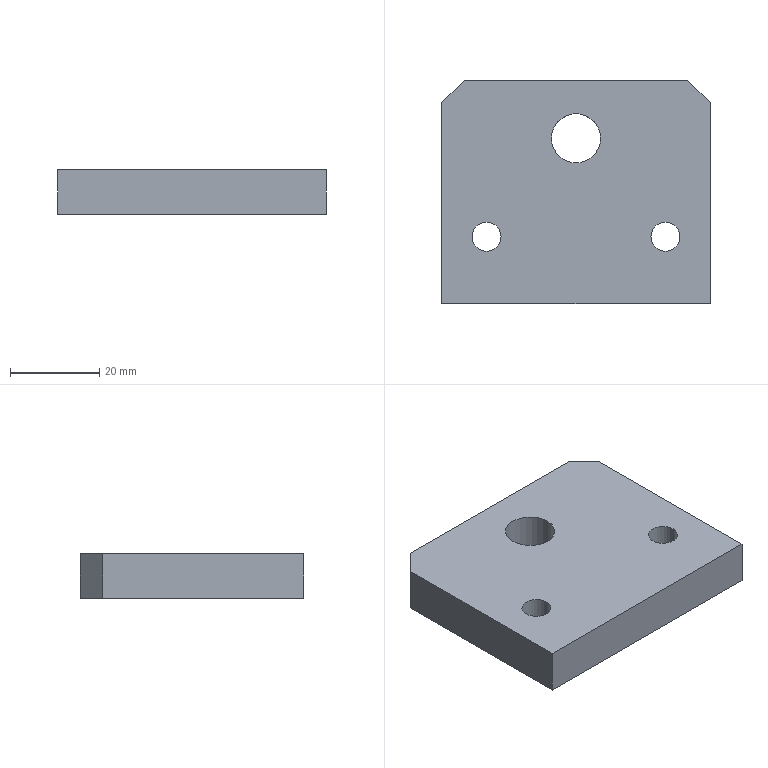Part | SolidWorks | features Cut 2, Chamfer 1, Extrusion 1 | 1 solid | 14 faces | box 60 x 50 x 10 mm | volume 28136 mm3 | plane 8 | cylinder 6 | commonest cylinder face diameters 6.5 x4 11 x2
STEP:
#1=CARTESIAN_POINT('',(-21.994,-12.765,10.));
#2=VERTEX_POINT('',#1);
#3=CARTESIAN_POINT('',(-28.494,-12.765,10.));
#4=VERTEX_POINT('',#3);
#5=CARTESIAN_POINT('',(-25.244,-12.765,10.));
#6=DIRECTION('',(0.,0.,-1.));
#7=DIRECTION('',(-1.,0.,0.));
#8=AXIS2_PLACEMENT_3D('',#5,#6,#7);
#9=CIRCLE('',#8,3.25);
#10=EDGE_CURVE('',#2,#4,#9,.T.);
#11=ORIENTED_EDGE('',*,*,#10,.F.);
#12=CARTESIAN_POINT('',(-21.994,-12.765,0.));
#13=VERTEX_POINT('',#12);
#14=CARTESIAN_POINT('',(-21.994,-12.765,10.));
#15=DIRECTION('',(0.,0.,-1.));
#16=VECTOR('',#15,1000.);
#17=LINE('',#14,#16);
#18=EDGE_CURVE('',#2,#13,#17,.T.);
#19=ORIENTED_EDGE('',*,*,#18,.T.);
#20=CARTESIAN_POINT('',(-28.494,-12.765,0.));
#21=VERTEX_POINT('',#20);
#22=CARTESIAN_POINT('',(-25.244,-12.765,0.));
#23=DIRECTION('',(0.,0.,-1.));
#24=DIRECTION('',(-1.,0.,0.));
#25=AXIS2_PLACEMENT_3D('',#22,#23,#24);
#26=CIRCLE('',#25,3.25);
#27=EDGE_CURVE('',#13,#21,#26,.T.);
#28=ORIENTED_EDGE('',*,*,#27,.T.);
#29=CARTESIAN_POINT('',(-28.494,-12.765,10.));
#30=DIRECTION('',(0.,0.,-1.));
#31=VECTOR('',#30,1000.);
#32=LINE('',#29,#31);
#33=EDGE_CURVE('',#4,#21,#32,.T.);
#34=ORIENTED_EDGE('',*,*,#33,.F.);
#35=EDGE_LOOP('',(#11,#19,#28,#34));
#36=FACE_OUTER_BOUND('',#35,.T.);
#37=CARTESIAN_POINT('',(-25.244,-12.765,10.));
#38=DIRECTION('',(0.,0.,-1.));
#39=DIRECTION('',(-1.,0.,0.));
#40=AXIS2_PLACEMENT_3D('',#37,#38,#39);
#41=CYLINDRICAL_SURFACE('',#40,3.25);
#42=ADVANCED_FACE('',(#36),#41,.F.);
#43=CARTESIAN_POINT('',(18.006,-12.765,10.));
#44=VERTEX_POINT('',#43);
#45=CARTESIAN_POINT('',(11.506,-12.765,10.));
#46=VERTEX_POINT('',#45);
#47=CARTESIAN_POINT('',(14.756,-12.765,10.));
#48=DIRECTION('',(0.,0.,-1.));
#49=DIRECTION('',(-1.,0.,0.));
#50=AXIS2_PLACEMENT_3D('',#47,#48,#49);
#51=CIRCLE('',#50,3.25);
#52=EDGE_CURVE('',#44,#46,#51,.T.);
#53=ORIENTED_EDGE('',*,*,#52,.F.);
#54=CARTESIAN_POINT('',(18.006,-12.765,0.));
#55=VERTEX_POINT('',#54);
#56=CARTESIAN_POINT('',(18.006,-12.765,10.));
#57=DIRECTION('',(0.,0.,-1.));
#58=VECTOR('',#57,1000.);
#59=LINE('',#56,#58);
#60=EDGE_CURVE('',#44,#55,#59,.T.);
#61=ORIENTED_EDGE('',*,*,#60,.T.);
#62=CARTESIAN_POINT('',(11.506,-12.765,0.));
#63=VERTEX_POINT('',#62);
#64=CARTESIAN_POINT('',(14.756,-12.765,0.));
#65=DIRECTION('',(0.,0.,-1.));
#66=DIRECTION('',(-1.,0.,0.));
#67=AXIS2_PLACEMENT_3D('',#64,#65,#66);
#68=CIRCLE('',#67,3.25);
#69=EDGE_CURVE('',#55,#63,#68,.T.);
#70=ORIENTED_EDGE('',*,*,#69,.T.);
#71=CARTESIAN_POINT('',(11.506,-12.765,10.));
#72=DIRECTION('',(0.,0.,-1.));
#73=VECTOR('',#72,1000.);
#74=LINE('',#71,#73);
#75=EDGE_CURVE('',#46,#63,#74,.T.);
#76=ORIENTED_EDGE('',*,*,#75,.F.);
#77=EDGE_LOOP('',(#53,#61,#70,#76));
#78=FACE_OUTER_BOUND('',#77,.T.);
#79=CARTESIAN_POINT('',(14.756,-12.765,10.));
#80=DIRECTION('',(0.,0.,-1.));
#81=DIRECTION('',(-1.,0.,0.));
#82=AXIS2_PLACEMENT_3D('',#79,#80,#81);
#83=CYLINDRICAL_SURFACE('',#82,3.25);
#84=ADVANCED_FACE('',(#78),#83,.F.);
#85=CARTESIAN_POINT('',(-10.744,9.235,10.));
#86=VERTEX_POINT('',#85);
#87=CARTESIAN_POINT('',(0.2561,9.235,10.));
#88=VERTEX_POINT('',#87);
#89=CARTESIAN_POINT('',(-5.244,9.235,10.));
#90=DIRECTION('',(0.,0.,1.));
#91=DIRECTION('',(1.,0.,0.));
#92=AXIS2_PLACEMENT_3D('',#89,#90,#91);
#93=CIRCLE('',#92,5.5);
#94=EDGE_CURVE('',#86,#88,#93,.T.);
#95=ORIENTED_EDGE('',*,*,#94,.T.);
#96=CARTESIAN_POINT('',(0.2561,9.235,0.));
#97=VERTEX_POINT('',#96);
#98=CARTESIAN_POINT('',(0.2561,9.235,18.));
#99=DIRECTION('',(0.,0.,-1.));
#100=VECTOR('',#99,1000.);
#101=LINE('',#98,#100);
#102=EDGE_CURVE('',#88,#97,#101,.T.);
#103=ORIENTED_EDGE('',*,*,#102,.T.);
#104=CARTESIAN_POINT('',(-10.744,9.235,0.));
#105=VERTEX_POINT('',#104);
#106=CARTESIAN_POINT('',(-5.244,9.235,0.));
#107=DIRECTION('',(0.,0.,-1.));
#108=DIRECTION('',(-1.,0.,0.));
#109=AXIS2_PLACEMENT_3D('',#106,#107,#108);
#110=CIRCLE('',#109,5.5);
#111=EDGE_CURVE('',#97,#105,#110,.T.);
#112=ORIENTED_EDGE('',*,*,#111,.T.);
#113=CARTESIAN_POINT('',(-10.744,9.235,18.));
#114=DIRECTION('',(0.,0.,-1.));
#115=VECTOR('',#114,1000.);
#116=LINE('',#113,#115);
#117=EDGE_CURVE('',#86,#105,#116,.T.);
#118=ORIENTED_EDGE('',*,*,#117,.F.);
#119=EDGE_LOOP('',(#95,#103,#112,#118));
#120=FACE_OUTER_BOUND('',#119,.T.);
#121=CARTESIAN_POINT('',(-5.244,9.235,18.));
#122=DIRECTION('',(0.,0.,-1.));
#123=DIRECTION('',(-1.,0.,0.));
#124=AXIS2_PLACEMENT_3D('',#121,#122,#123);
#125=CYLINDRICAL_SURFACE('',#124,5.5);
#126=ADVANCED_FACE('',(#120),#125,.F.);
#127=CARTESIAN_POINT('',(-35.244,17.235,10.));
#128=VERTEX_POINT('',#127);
#129=CARTESIAN_POINT('',(-35.244,-27.765,10.));
#130=VERTEX_POINT('',#129);
#131=CARTESIAN_POINT('',(-35.244,22.235,10.));
#132=DIRECTION('',(0.,-1.,0.));
#133=VECTOR('',#132,1000.);
#134=LINE('',#131,#133);
#135=EDGE_CURVE('',#128,#130,#134,.T.);
#136=ORIENTED_EDGE('',*,*,#135,.F.);
#137=CARTESIAN_POINT('',(-35.244,17.235,0.));
#138=VERTEX_POINT('',#137);
#139=CARTESIAN_POINT('',(-35.244,17.235,10.));
#140=DIRECTION('',(0.,0.,-1.));
#141=VECTOR('',#140,1000.);
#142=LINE('',#139,#141);
#143=EDGE_CURVE('',#128,#138,#142,.T.);
#144=ORIENTED_EDGE('',*,*,#143,.T.);
#145=CARTESIAN_POINT('',(-35.244,-27.765,0.));
#146=VERTEX_POINT('',#145);
#147=CARTESIAN_POINT('',(-35.244,22.235,0.));
#148=DIRECTION('',(0.,-1.,0.));
#149=VECTOR('',#148,1000.);
#150=LINE('',#147,#149);
#151=EDGE_CURVE('',#138,#146,#150,.T.);
#152=ORIENTED_EDGE('',*,*,#151,.T.);
#153=CARTESIAN_POINT('',(-35.244,-27.765,10.));
#154=DIRECTION('',(0.,0.,-1.));
#155=VECTOR('',#154,1000.);
#156=LINE('',#153,#155);
#157=EDGE_CURVE('',#130,#146,#156,.T.);
#158=ORIENTED_EDGE('',*,*,#157,.F.);
#159=EDGE_LOOP('',(#136,#144,#152,#158));
#160=FACE_OUTER_BOUND('',#159,.T.);
#161=CARTESIAN_POINT('',(-35.244,22.235,10.));
#162=DIRECTION('',(1.,0.,0.));
#163=DIRECTION('',(0.,0.,-1.));
#164=AXIS2_PLACEMENT_3D('',#161,#162,#163);
#165=PLANE('',#164);
#166=ADVANCED_FACE('',(#160),#165,.F.);
#167=CARTESIAN_POINT('',(24.756,-27.765,0.));
#168=VERTEX_POINT('',#167);
#169=CARTESIAN_POINT('',(-35.244,-27.765,0.));
#170=DIRECTION('',(1.,0.,0.));
#171=VECTOR('',#170,1000.);
#172=LINE('',#169,#171);
#173=EDGE_CURVE('',#146,#168,#172,.T.);
#174=ORIENTED_EDGE('',*,*,#173,.T.);
#175=CARTESIAN_POINT('',(24.756,-27.765,10.));
#176=VERTEX_POINT('',#175);
#177=CARTESIAN_POINT('',(24.756,-27.765,10.));
#178=DIRECTION('',(0.,0.,-1.));
#179=VECTOR('',#178,1000.);
#180=LINE('',#177,#179);
#181=EDGE_CURVE('',#176,#168,#180,.T.);
#182=ORIENTED_EDGE('',*,*,#181,.F.);
#183=CARTESIAN_POINT('',(-35.244,-27.765,10.));
#184=DIRECTION('',(1.,0.,0.));
#185=VECTOR('',#184,1000.);
#186=LINE('',#183,#185);
#187=EDGE_CURVE('',#130,#176,#186,.T.);
#188=ORIENTED_EDGE('',*,*,#187,.F.);
#189=ORIENTED_EDGE('',*,*,#157,.T.);
#190=EDGE_LOOP('',(#174,#182,#188,#189));
#191=FACE_OUTER_BOUND('',#190,.T.);
#192=CARTESIAN_POINT('',(-35.244,-27.765,10.));
#193=DIRECTION('',(0.,1.,0.));
#194=DIRECTION('',(0.,0.,1.));
#195=AXIS2_PLACEMENT_3D('',#192,#193,#194);
#196=PLANE('',#195);
#197=ADVANCED_FACE('',(#191),#196,.F.);
#198=CARTESIAN_POINT('',(24.756,17.235,0.));
#199=VERTEX_POINT('',#198);
#200=CARTESIAN_POINT('',(24.756,22.235,0.));
#201=DIRECTION('',(0.,1.,0.));
#202=VECTOR('',#201,1000.);
#203=LINE('',#200,#202);
#204=EDGE_CURVE('',#168,#199,#203,.T.);
#205=ORIENTED_EDGE('',*,*,#204,.T.);
#206=CARTESIAN_POINT('',(24.756,17.235,10.));
#207=VERTEX_POINT('',#206);
#208=CARTESIAN_POINT('',(24.756,17.235,10.));
#209=DIRECTION('',(0.,0.,1.));
#210=VECTOR('',#209,1000.);
#211=LINE('',#208,#210);
#212=EDGE_CURVE('',#199,#207,#211,.T.);
#213=ORIENTED_EDGE('',*,*,#212,.T.);
#214=CARTESIAN_POINT('',(24.756,22.235,10.));
#215=DIRECTION('',(0.,1.,0.));
#216=VECTOR('',#215,1000.);
#217=LINE('',#214,#216);
#218=EDGE_CURVE('',#176,#207,#217,.T.);
#219=ORIENTED_EDGE('',*,*,#218,.F.);
#220=ORIENTED_EDGE('',*,*,#181,.T.);
#221=EDGE_LOOP('',(#205,#213,#219,#220));
#222=FACE_OUTER_BOUND('',#221,.T.);
#223=CARTESIAN_POINT('',(24.756,22.235,10.));
#224=DIRECTION('',(-1.,0.,0.));
#225=DIRECTION('',(0.,-1.,0.));
#226=AXIS2_PLACEMENT_3D('',#223,#224,#225);
#227=PLANE('',#226);
#228=ADVANCED_FACE('',(#222),#227,.F.);
#229=CARTESIAN_POINT('',(19.756,22.235,0.));
#230=VERTEX_POINT('',#229);
#231=CARTESIAN_POINT('',(-30.244,22.235,0.));
#232=VERTEX_POINT('',#231);
#233=CARTESIAN_POINT('',(-35.244,22.235,0.));
#234=DIRECTION('',(-1.,0.,0.));
#235=VECTOR('',#234,1000.);
#236=LINE('',#233,#235);
#237=EDGE_CURVE('',#230,#232,#236,.T.);
#238=ORIENTED_EDGE('',*,*,#237,.T.);
#239=CARTESIAN_POINT('',(-30.244,22.235,10.));
#240=VERTEX_POINT('',#239);
#241=CARTESIAN_POINT('',(-30.244,22.235,10.));
#242=DIRECTION('',(0.,0.,1.));
#243=VECTOR('',#242,1000.);
#244=LINE('',#241,#243);
#245=EDGE_CURVE('',#232,#240,#244,.T.);
#246=ORIENTED_EDGE('',*,*,#245,.T.);
#247=CARTESIAN_POINT('',(19.756,22.235,10.));
#248=VERTEX_POINT('',#247);
#249=CARTESIAN_POINT('',(-35.244,22.235,10.));
#250=DIRECTION('',(-1.,0.,0.));
#251=VECTOR('',#250,1000.);
#252=LINE('',#249,#251);
#253=EDGE_CURVE('',#248,#240,#252,.T.);
#254=ORIENTED_EDGE('',*,*,#253,.F.);
#255=CARTESIAN_POINT('',(19.756,22.235,10.));
#256=DIRECTION('',(0.,0.,-1.));
#257=VECTOR('',#256,1000.);
#258=LINE('',#255,#257);
#259=EDGE_CURVE('',#248,#230,#258,.T.);
#260=ORIENTED_EDGE('',*,*,#259,.T.);
#261=EDGE_LOOP('',(#238,#246,#254,#260));
#262=FACE_OUTER_BOUND('',#261,.T.);
#263=CARTESIAN_POINT('',(-35.244,22.235,10.));
#264=DIRECTION('',(0.,-1.,0.));
#265=DIRECTION('',(0.,0.,-1.));
#266=AXIS2_PLACEMENT_3D('',#263,#264,#265);
#267=PLANE('',#266);
#268=ADVANCED_FACE('',(#262),#267,.F.);
#269=CARTESIAN_POINT('',(-25.244,-12.765,10.));
#270=DIRECTION('',(0.,0.,-1.));
#271=DIRECTION('',(-1.,0.,0.));
#272=AXIS2_PLACEMENT_3D('',#269,#270,#271);
#273=CIRCLE('',#272,3.25);
#274=EDGE_CURVE('',#4,#2,#273,.T.);
#275=ORIENTED_EDGE('',*,*,#274,.T.);
#276=ORIENTED_EDGE('',*,*,#10,.T.);
#277=EDGE_LOOP('',(#275,#276));
#278=FACE_BOUND('',#277,.T.);
#279=CARTESIAN_POINT('',(14.756,-12.765,10.));
#280=DIRECTION('',(0.,0.,-1.));
#281=DIRECTION('',(-1.,0.,0.));
#282=AXIS2_PLACEMENT_3D('',#279,#280,#281);
#283=CIRCLE('',#282,3.25);
#284=EDGE_CURVE('',#46,#44,#283,.T.);
#285=ORIENTED_EDGE('',*,*,#284,.T.);
#286=ORIENTED_EDGE('',*,*,#52,.T.);
#287=EDGE_LOOP('',(#285,#286));
#288=FACE_BOUND('',#287,.T.);
#289=ORIENTED_EDGE('',*,*,#94,.F.);
#290=CARTESIAN_POINT('',(-5.244,9.235,10.));
#291=DIRECTION('',(0.,0.,1.));
#292=DIRECTION('',(1.,0.,0.));
#293=AXIS2_PLACEMENT_3D('',#290,#291,#292);
#294=CIRCLE('',#293,5.5);
#295=EDGE_CURVE('',#88,#86,#294,.T.);
#296=ORIENTED_EDGE('',*,*,#295,.F.);
#297=EDGE_LOOP('',(#289,#296));
#298=FACE_BOUND('',#297,.T.);
#299=ORIENTED_EDGE('',*,*,#253,.T.);
#300=CARTESIAN_POINT('',(-26.239,26.239,10.));
#301=DIRECTION('',(-0.7071,-0.7071,0.));
#302=VECTOR('',#301,1000.);
#303=LINE('',#300,#302);
#304=EDGE_CURVE('',#240,#128,#303,.T.);
#305=ORIENTED_EDGE('',*,*,#304,.T.);
#306=ORIENTED_EDGE('',*,*,#135,.T.);
#307=ORIENTED_EDGE('',*,*,#187,.T.);
#308=ORIENTED_EDGE('',*,*,#218,.T.);
#309=CARTESIAN_POINT('',(20.995,20.995,10.));
#310=DIRECTION('',(-0.7071,0.7071,0.));
#311=VECTOR('',#310,1000.);
#312=LINE('',#309,#311);
#313=EDGE_CURVE('',#207,#248,#312,.T.);
#314=ORIENTED_EDGE('',*,*,#313,.T.);
#315=EDGE_LOOP('',(#299,#305,#306,#307,#308,#314));
#316=FACE_OUTER_BOUND('',#315,.T.);
#317=CARTESIAN_POINT('',(0.,0.,10.));
#318=DIRECTION('',(0.,0.,1.));
#319=DIRECTION('',(1.,0.,0.));
#320=AXIS2_PLACEMENT_3D('',#317,#318,#319);
#321=PLANE('',#320);
#322=ADVANCED_FACE('',(#278,#288,#298,#316),#321,.T.);
#323=CARTESIAN_POINT('',(-25.244,-12.765,0.));
#324=DIRECTION('',(0.,0.,-1.));
#325=DIRECTION('',(-1.,0.,0.));
#326=AXIS2_PLACEMENT_3D('',#323,#324,#325);
#327=CIRCLE('',#326,3.25);
#328=EDGE_CURVE('',#21,#13,#327,.T.);
#329=ORIENTED_EDGE('',*,*,#328,.F.);
#330=ORIENTED_EDGE('',*,*,#27,.F.);
#331=EDGE_LOOP('',(#329,#330));
#332=FACE_BOUND('',#331,.T.);
#333=CARTESIAN_POINT('',(14.756,-12.765,0.));
#334=DIRECTION('',(0.,0.,-1.));
#335=DIRECTION('',(-1.,0.,0.));
#336=AXIS2_PLACEMENT_3D('',#333,#334,#335);
#337=CIRCLE('',#336,3.25);
#338=EDGE_CURVE('',#63,#55,#337,.T.);
#339=ORIENTED_EDGE('',*,*,#338,.F.);
#340=ORIENTED_EDGE('',*,*,#69,.F.);
#341=EDGE_LOOP('',(#339,#340));
#342=FACE_BOUND('',#341,.T.);
#343=CARTESIAN_POINT('',(-5.244,9.235,0.));
#344=DIRECTION('',(0.,0.,-1.));
#345=DIRECTION('',(-1.,0.,0.));
#346=AXIS2_PLACEMENT_3D('',#343,#344,#345);
#347=CIRCLE('',#346,5.5);
#348=EDGE_CURVE('',#105,#97,#347,.T.);
#349=ORIENTED_EDGE('',*,*,#348,.F.);
#350=ORIENTED_EDGE('',*,*,#111,.F.);
#351=EDGE_LOOP('',(#349,#350));
#352=FACE_BOUND('',#351,.T.);
#353=ORIENTED_EDGE('',*,*,#151,.F.);
#354=CARTESIAN_POINT('',(-35.244,17.235,0.));
#355=DIRECTION('',(0.7071,0.7071,0.));
#356=VECTOR('',#355,1000.);
#357=LINE('',#354,#356);
#358=EDGE_CURVE('',#138,#232,#357,.T.);
#359=ORIENTED_EDGE('',*,*,#358,.T.);
#360=ORIENTED_EDGE('',*,*,#237,.F.);
#361=CARTESIAN_POINT('',(19.756,22.235,0.));
#362=DIRECTION('',(0.7071,-0.7071,0.));
#363=VECTOR('',#362,1000.);
#364=LINE('',#361,#363);
#365=EDGE_CURVE('',#230,#199,#364,.T.);
#366=ORIENTED_EDGE('',*,*,#365,.T.);
#367=ORIENTED_EDGE('',*,*,#204,.F.);
#368=ORIENTED_EDGE('',*,*,#173,.F.);
#369=EDGE_LOOP('',(#353,#359,#360,#366,#367,#368));
#370=FACE_OUTER_BOUND('',#369,.T.);
#371=CARTESIAN_POINT('',(0.,0.,0.));
#372=DIRECTION('',(0.,0.,1.));
#373=DIRECTION('',(1.,0.,0.));
#374=AXIS2_PLACEMENT_3D('',#371,#372,#373);
#375=PLANE('',#374);
#376=ADVANCED_FACE('',(#332,#342,#352,#370),#375,.F.);
#377=ORIENTED_EDGE('',*,*,#102,.F.);
#378=ORIENTED_EDGE('',*,*,#295,.T.);
#379=ORIENTED_EDGE('',*,*,#117,.T.);
#380=ORIENTED_EDGE('',*,*,#348,.T.);
#381=EDGE_LOOP('',(#377,#378,#379,#380));
#382=FACE_OUTER_BOUND('',#381,.T.);
#383=CARTESIAN_POINT('',(-5.244,9.235,18.));
#384=DIRECTION('',(0.,0.,-1.));
#385=DIRECTION('',(-1.,0.,0.));
#386=AXIS2_PLACEMENT_3D('',#383,#384,#385);
#387=CYLINDRICAL_SURFACE('',#386,5.5);
#388=ADVANCED_FACE('',(#382),#387,.F.);
#389=ORIENTED_EDGE('',*,*,#304,.F.);
#390=ORIENTED_EDGE('',*,*,#245,.F.);
#391=ORIENTED_EDGE('',*,*,#358,.F.);
#392=ORIENTED_EDGE('',*,*,#143,.F.);
#393=EDGE_LOOP('',(#389,#390,#391,#392));
#394=FACE_OUTER_BOUND('',#393,.T.);
#395=CARTESIAN_POINT('',(-35.244,17.235,10.));
#396=DIRECTION('',(0.7071,-0.7071,0.));
#397=DIRECTION('',(0.,0.,-1.));
#398=AXIS2_PLACEMENT_3D('',#395,#396,#397);
#399=PLANE('',#398);
#400=ADVANCED_FACE('',(#394),#399,.F.);
#401=ORIENTED_EDGE('',*,*,#313,.F.);
#402=ORIENTED_EDGE('',*,*,#212,.F.);
#403=ORIENTED_EDGE('',*,*,#365,.F.);
#404=ORIENTED_EDGE('',*,*,#259,.F.);
#405=EDGE_LOOP('',(#401,#402,#403,#404));
#406=FACE_OUTER_BOUND('',#405,.T.);
#407=CARTESIAN_POINT('',(19.756,22.235,10.));
#408=DIRECTION('',(-0.7071,-0.7071,0.));
#409=DIRECTION('',(0.,0.,-1.));
#410=AXIS2_PLACEMENT_3D('',#407,#408,#409);
#411=PLANE('',#410);
#412=ADVANCED_FACE('',(#406),#411,.F.);
#413=ORIENTED_EDGE('',*,*,#60,.F.);
#414=ORIENTED_EDGE('',*,*,#284,.F.);
#415=ORIENTED_EDGE('',*,*,#75,.T.);
#416=ORIENTED_EDGE('',*,*,#338,.T.);
#417=EDGE_LOOP('',(#413,#414,#415,#416));
#418=FACE_OUTER_BOUND('',#417,.T.);
#419=CARTESIAN_POINT('',(14.756,-12.765,10.));
#420=DIRECTION('',(0.,0.,-1.));
#421=DIRECTION('',(-1.,0.,0.));
#422=AXIS2_PLACEMENT_3D('',#419,#420,#421);
#423=CYLINDRICAL_SURFACE('',#422,3.25);
#424=ADVANCED_FACE('',(#418),#423,.F.);
#425=ORIENTED_EDGE('',*,*,#18,.F.);
#426=ORIENTED_EDGE('',*,*,#274,.F.);
#427=ORIENTED_EDGE('',*,*,#33,.T.);
#428=ORIENTED_EDGE('',*,*,#328,.T.);
#429=EDGE_LOOP('',(#425,#426,#427,#428));
#430=FACE_OUTER_BOUND('',#429,.T.);
#431=CARTESIAN_POINT('',(-25.244,-12.765,10.));
#432=DIRECTION('',(0.,0.,-1.));
#433=DIRECTION('',(-1.,0.,0.));
#434=AXIS2_PLACEMENT_3D('',#431,#432,#433);
#435=CYLINDRICAL_SURFACE('',#434,3.25);
#436=ADVANCED_FACE('',(#430),#435,.F.);
#437=CLOSED_SHELL('',(#42,#84,#126,#166,#197,#228,#268,#322,#376,#388,#400,#412,#424,#436));
#438=MANIFOLD_SOLID_BREP('',#437);
#439=CARTESIAN_POINT('',(0.,0.,0.));
#440=DIRECTION('',(0.,0.,1.));
#441=DIRECTION('',(1.,0.,0.));
#442=AXIS2_PLACEMENT_3D('',#439,#440,#441);
#443=(LENGTH_UNIT()NAMED_UNIT(*)SI_UNIT(.MILLI.,.METRE.));
#444=UNCERTAINTY_MEASURE_WITH_UNIT(LENGTH_MEASURE(0.00001),#443,'','');
#445=(NAMED_UNIT(*)PLANE_ANGLE_UNIT()SI_UNIT($,.RADIAN.));
#446=(NAMED_UNIT(*)SI_UNIT($,.STERADIAN.)SOLID_ANGLE_UNIT());
#447=(GEOMETRIC_REPRESENTATION_CONTEXT(3)GLOBAL_UNCERTAINTY_ASSIGNED_CONTEXT((#444))GLOBAL_UNIT_ASSIGNED_CONTEXT((#443,#445,#446))REPRESENTATION_CONTEXT('',''));
#448=ADVANCED_BREP_SHAPE_REPRESENTATION('',(#438,#442),#447);